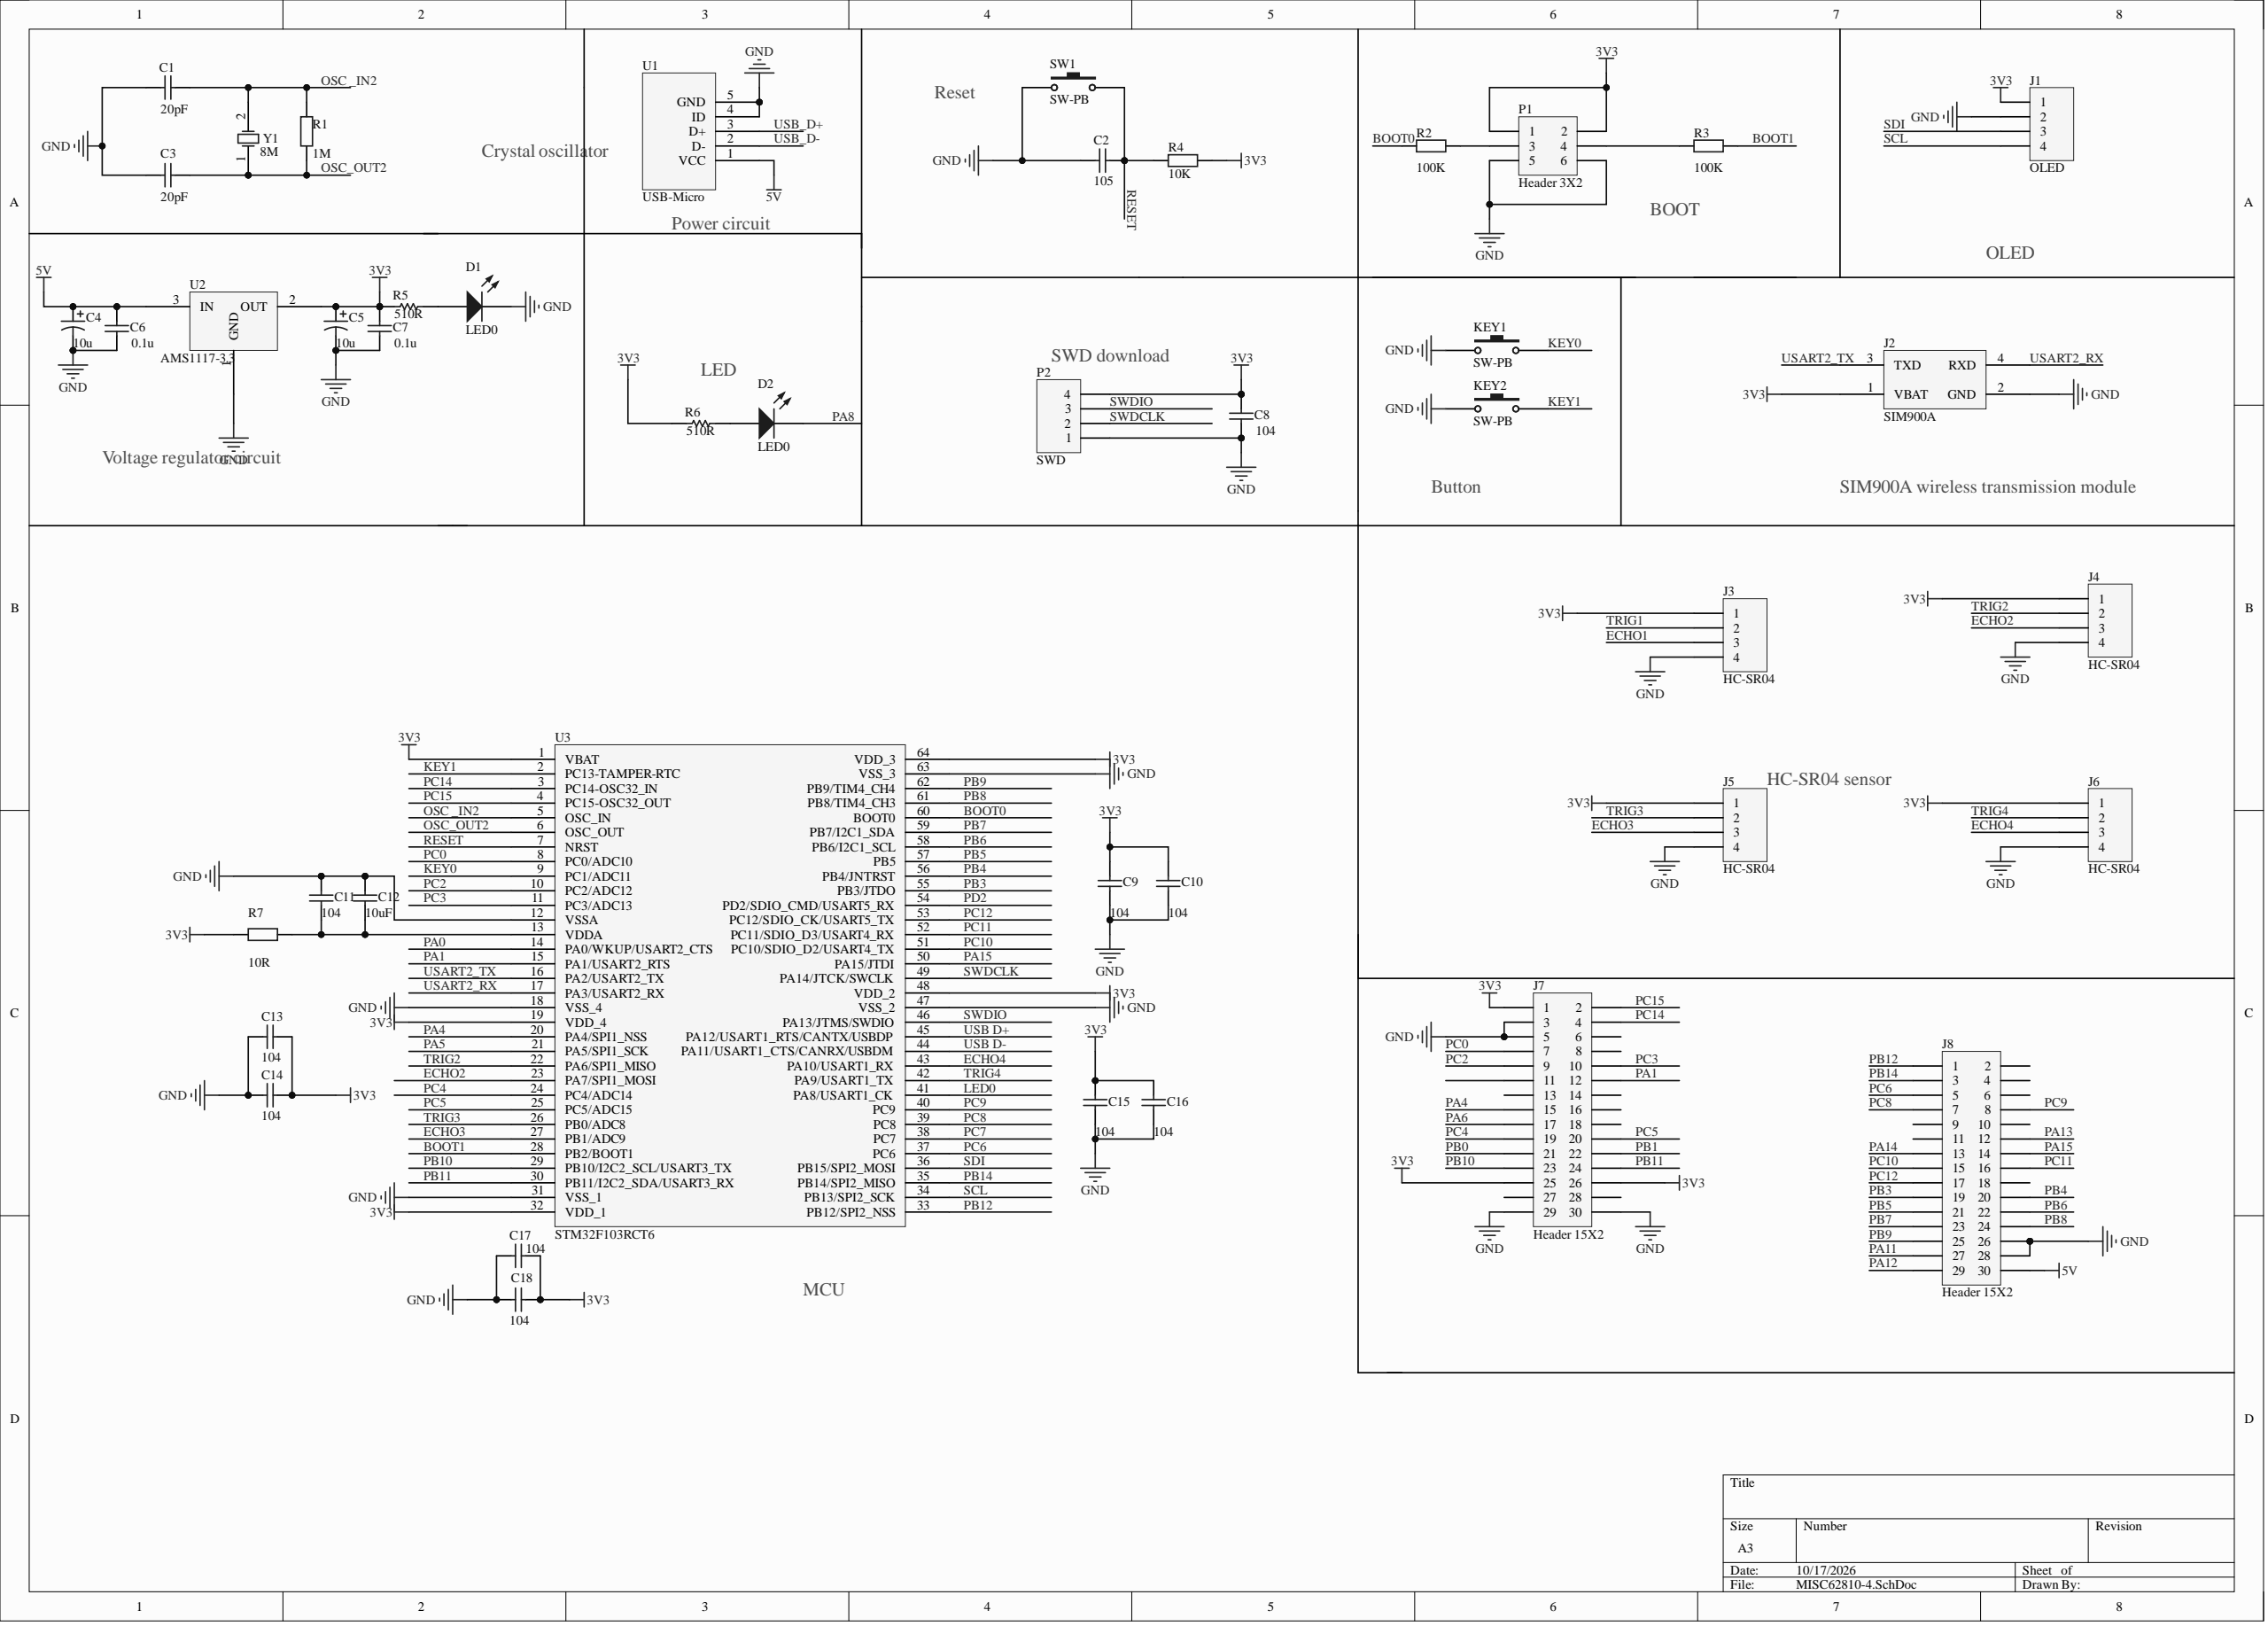Circuit board | Altium Designer | 44 parts | 54 nets
Bill of materials:
Comment,Description,Designator,Footprint,LibRef,Quantity
"Cap","Capacitor","C1, C3, C6, C7, C8, C9, C10, C11, C12, C13, C14, C15, C16, C17, C18","C 0805_L","Cap","15"
"","Capacitor","C2","C 0805_L","Cap","1"
"Cap Pol1","Polarized Capacitor (Radial)","C4, C5","CM A(3*5.4)","Cap Pol1","2"
"LED0","Typical INFRARED GaAs LED","D1, D2","LED 0805G","LED0","2"
"OLED","Header, 4-Pin","J1","0.96OLED_4P","Header 4","1"
"SIM900A","","J2","HDR1X4","Component_1","1"
"HC-SR04","Header, 4-Pin","J3, J4, J5, J6","HDR1X4","Header 4","4"
"Header 15X2","Header, 15-Pin, Dual row","J7, J8","HDR2X15","Header 15X2","2"
"SW-PB","Switch","KEY1, KEY2, SW1","TSW SMD-3*4*2.5","SW-PB","3"
"Header 3X2","Header, 3-Pin, Dual row","P1","HDR2X3","Header 3X2","1"
"SWD","Header, 4-Pin","P2","HDR1X4","Header 4","1"
"","Resistor","R1","R 0805_L","Res2","1"
"Res2","Resistor","R2, R3, R4, R7","R 0805_L","Res2","4"
"Res1","Resistor","R5, R6","R 0805_L","Res1","2"
"USB-Micro","","U1","USB-MICRO_B","Component_1","1"
"AMS1117-3.3","","U2","SOT223","Component_1","1"
"STM32F103RCT6","","U3","LQFP64 7x7","Component_1","1"
"8M","Crystal Oscillator","Y1","OSC 5032-2P","XTAL","1"
Netlist (Protel format):
[
C1
C 0805_L
Cap



]
[
C2
C 0805_L




]
[
C3
C 0805_L
Cap



]
[
C4
CM A(3*5.4)
Cap Pol1



]
[
C5
CM A(3*5.4)
Cap Pol1



]
[
C6
C 0805_L
Cap



]
[
C7
C 0805_L
Cap



]
[
C8
C 0805_L
Cap



]
[
C9
C 0805_L
Cap



]
[
C10
C 0805_L
Cap



]
[
C11
C 0805_L
Cap



]
[
C12
C 0805_L
Cap



]
[
C13
C 0805_L
Cap



]
[
C14
C 0805_L
Cap



]
[
C15
C 0805_L
Cap



]
[
C16
C 0805_L
Cap



]
[
C17
C 0805_L
Cap



]
[
C18
C 0805_L
Cap



]
[
D1
LED 0805G
LED0



]
[
D2
LED 0805G
LED0



]
[
J1
0.96OLED_4P
OLED



]
[
J2
HDR1X4
SIM900A



]
[
J3
HDR1X4
HC-SR04



]
[
J4
HDR1X4
HC-SR04



]
[
J5
HDR1X4
HC-SR04



]
[
J6
HDR1X4
HC-SR04



]
[
J7
HDR2X15
Header 15X2



]
[
J8
HDR2X15
Header 15X2



]
[
KEY1
TSW SMD-3*4*2.5
SW-PB



]
[
KEY2
TSW SMD-3*4*2.5
SW-PB



]
[
P1
HDR2X3
Header 3X2



]
[
P2
HDR1X4
SWD



]
[
R1
R 0805_L




]
[
R2
R 0805_L
Res2



]
[
R3
R 0805_L
Res2



]
[
R4
R 0805_L
Res2



]
[
R5
R 0805_L
Res1



]
[
R6
R 0805_L
Res1



]
[
R7
R 0805_L
Res2



]
[
SW1
TSW SMD-3*4*2.5
SW-PB



]
[
U1
USB-MICRO_B
USB-Micro



]
[
U2
SOT223
AMS1117-3.3



]
[
U3
LQFP64 7x7
STM32F103RCT6



]
[
Y1
OSC 5032-2P
8M



]
(
USART2_TX
J2-3
U3-16
)
(
USART2_RX
J2-4
U3-17
)
(
TRIG4
J6-2
U3-42
)
(
TRIG3
J5-2
U3-26
)
(
TRIG2
J4-2
U3-22
)
(
SWDIO
P2-3
U3-46
)
(
SWDCLK
P2-2
U3-49
)
(
SDI
J1-3
U3-36
)
(
SCL
J1-4
U3-34
)
(
RESET
C2-2
R4-1
SW1-2
U3-7
)
(
PC15
J7-2
U3-4
)
(
PC14
J7-4
U3-3
)
(
PC12
J8-17
U3-53
)
(
PC11
J8-16
U3-52
)
(
PC10
J8-15
U3-51
)
(
PC9
J8-8
U3-40
)
(
PC8
J8-7
U3-39
)
(
PC6
J8-5
U3-37
)
(
PC5
J7-20
U3-25
)
(
PC4
J7-19
U3-24
)
(
PC3
J7-10
U3-11
)
(
PC2
J7-9
U3-10
)
(
PC0
J7-7
U3-8
)
(
PB14
J8-3
U3-35
)
(
PB12
J8-1
U3-33
)
(
PB11
J7-24
U3-30
)
(
PB10
J7-23
U3-29
)
(
PB9
J8-25
U3-62
)
(
PB8
J8-24
U3-61
)
(
PB7
J8-23
U3-59
)
(
PB6
J8-22
U3-58
)
(
PB5
J8-21
U3-57
)
(
PB4
J8-20
U3-56
)
(
PB3
J8-19
U3-55
)
(
PA15
J8-14
U3-50
)
(
PA4
J7-15
U3-20
)
(
PA1
J7-12
U3-15
)
(
OSC_OUT2
C3-2
R1-1
U3-6
Y1-1
)
(
OSC _IN2
C1-2
R1-2
U3-5
Y1-2
)
(
NetP1_4
P1-4
R3-1
)
(
NetP1_3
P1-3
R2-2
)
(
NetD2_1
D2-1
R6-2
)
(
NetD1_1
D1-1
R5-2
)
(
NetC11_1
C11-1
C12-1
R7-2
U3-13
)
(
KEY1
KEY2-2
U3-2
)
(
KEY0
KEY1-2
U3-9
)
(
GND
C1-1
C2-1
C3-1
C4-2
C5-2
C6-1
C7-1
C8-1
C9-1
C10-1
C11-2
C12-2
C13-2
C14-2
C15-1
C16-1
C17-1
C18-1
D1-2
J1-2
J2-2
J3-4
J4-4
J5-4
J6-4
J7-3
J7-5
J7-29
J7-30
J8-26
J8-28
KEY1-1
KEY2-1
P1-5
P1-6
P2-1
SW1-1
U1-4
U1-5
U2-1
U3-12
U3-18
U3-31
U3-47
U3-63
)
(
ECHO4
J6-3
U3-43
)
(
ECHO3
J5-3
U3-27
)
(
ECHO2
J4-3
U3-23
)
(
BOOT1
R3-2
U3-28
)
(
BOOT0
R2-1
U3-60
)
(
5V
C4-1
C6-2
J8-30
U1-1
U2-3
)
(
3V3
C5-1
C7-2
C8-2
C9-2
C10-2
C13-1
C14-1
C15-2
C16-2
C17-2
C18-2
J1-1
J2-1
J3-1
J4-1
J5-1
J6-1
J7-1
J7-25
J7-26
P1-1
P1-2
P2-4
R4-2
R5-1
R6-1
R7-1
U2-2
U3-1
U3-19
U3-32
U3-48
U3-64
)